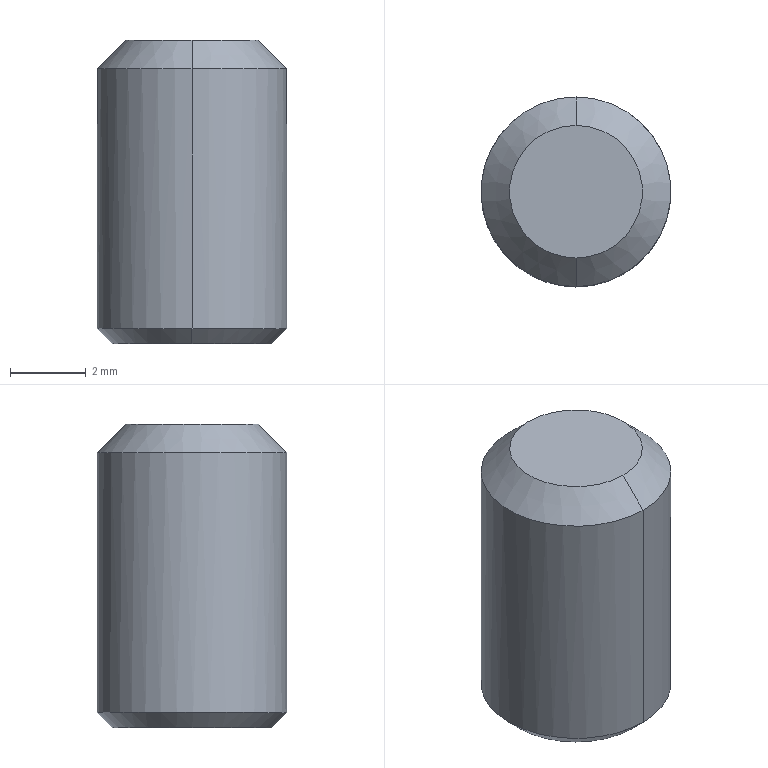Part | SolidWorks | features BaseBody 1 | 1 solid | 16 faces | box 5 x 5 x 8 mm | volume 135.67 mm3 | plane 10 | cone 4 | cylinder 2 | commonest cylinder face diameters 5 x2
STEP:
#1=CARTESIAN_POINT('',(483.507,-62.377,246.119));
#2=VERTEX_POINT('',#1);
#3=CARTESIAN_POINT('',(484.706,-62.684,246.118));
#4=VERTEX_POINT('',#3);
#5=CARTESIAN_POINT('',(483.507,-64.877,246.119));
#6=DIRECTION('',(-0.000000004,0.000000009,-1.));
#7=DIRECTION('',(0.,-1.,-0.000000009));
#8=AXIS2_PLACEMENT_3D('',#5,#6,#7);
#9=CIRCLE('',#8,2.5);
#10=EDGE_CURVE('',#2,#4,#9,.T.);
#11=ORIENTED_EDGE('',*,*,#10,.F.);
#12=CARTESIAN_POINT('',(483.507,-62.377,252.968));
#13=VERTEX_POINT('',#12);
#14=CARTESIAN_POINT('',(483.507,-62.377,249.543));
#15=DIRECTION('',(0.000000004,-0.000000009,1.));
#16=VECTOR('',#15,1000.);
#17=LINE('',#14,#16);
#18=EDGE_CURVE('',#2,#13,#17,.T.);
#19=ORIENTED_EDGE('',*,*,#18,.T.);
#20=CARTESIAN_POINT('',(483.507,-67.377,252.968));
#21=VERTEX_POINT('',#20);
#22=CARTESIAN_POINT('',(483.507,-64.877,252.968));
#23=DIRECTION('',(-0.000000004,0.000000009,-1.));
#24=DIRECTION('',(0.,-1.,-0.000000009));
#25=AXIS2_PLACEMENT_3D('',#22,#23,#24);
#26=CIRCLE('',#25,2.5);
#27=EDGE_CURVE('',#13,#21,#26,.T.);
#28=ORIENTED_EDGE('',*,*,#27,.T.);
#29=CARTESIAN_POINT('',(483.507,-67.377,246.118));
#30=VERTEX_POINT('',#29);
#31=CARTESIAN_POINT('',(483.507,-67.377,249.543));
#32=DIRECTION('',(0.000000004,-0.000000009,1.));
#33=VECTOR('',#32,1000.);
#34=LINE('',#31,#33);
#35=EDGE_CURVE('',#30,#21,#34,.T.);
#36=ORIENTED_EDGE('',*,*,#35,.F.);
#37=CARTESIAN_POINT('',(483.507,-64.877,246.118));
#38=DIRECTION('',(0.000000004,-0.000000009,1.));
#39=DIRECTION('',(0.,-1.,-0.000000009));
#40=AXIS2_PLACEMENT_3D('',#37,#38,#39);
#41=CIRCLE('',#40,2.5);
#42=EDGE_CURVE('',#30,#4,#41,.T.);
#43=ORIENTED_EDGE('',*,*,#42,.T.);
#44=EDGE_LOOP('',(#11,#19,#28,#36,#43));
#45=FACE_OUTER_BOUND('',#44,.T.);
#46=CARTESIAN_POINT('',(483.507,-64.877,249.543));
#47=DIRECTION('',(0.000000004,-0.000000009,1.));
#48=DIRECTION('',(0.,-1.,-0.000000009));
#49=AXIS2_PLACEMENT_3D('',#46,#47,#48);
#50=CYLINDRICAL_SURFACE('',#49,2.5);
#51=ADVANCED_FACE('',(#45),#50,.T.);
#52=CARTESIAN_POINT('',(483.507,-63.127,253.718));
#53=VERTEX_POINT('',#52);
#54=CARTESIAN_POINT('',(483.507,-66.627,253.718));
#55=VERTEX_POINT('',#54);
#56=CARTESIAN_POINT('',(483.507,-64.877,253.718));
#57=DIRECTION('',(-0.000000004,0.000000009,-1.));
#58=DIRECTION('',(0.,1.,0.000000009));
#59=AXIS2_PLACEMENT_3D('',#56,#57,#58);
#60=CIRCLE('',#59,1.75);
#61=EDGE_CURVE('',#53,#55,#60,.T.);
#62=ORIENTED_EDGE('',*,*,#61,.T.);
#63=CARTESIAN_POINT('',(483.507,-67.377,252.968));
#64=DIRECTION('',(-0.000000003,-0.7071,-0.7071));
#65=VECTOR('',#64,1000.);
#66=LINE('',#63,#65);
#67=EDGE_CURVE('',#55,#21,#66,.T.);
#68=ORIENTED_EDGE('',*,*,#67,.T.);
#69=ORIENTED_EDGE('',*,*,#27,.F.);
#70=CARTESIAN_POINT('',(483.507,-62.377,252.968));
#71=DIRECTION('',(-0.000000003,0.7071,-0.7071));
#72=VECTOR('',#71,1000.);
#73=LINE('',#70,#72);
#74=EDGE_CURVE('',#53,#13,#73,.T.);
#75=ORIENTED_EDGE('',*,*,#74,.F.);
#76=EDGE_LOOP('',(#62,#68,#69,#75));
#77=FACE_OUTER_BOUND('',#76,.T.);
#78=CARTESIAN_POINT('',(483.507,-64.877,252.968));
#79=DIRECTION('',(-0.000000004,0.000000009,-1.));
#80=DIRECTION('',(0.,1.,0.000000009));
#81=AXIS2_PLACEMENT_3D('',#78,#79,#80);
#82=CONICAL_SURFACE('',#81,2.5,0.7854);
#83=ADVANCED_FACE('',(#77),#82,.T.);
#84=CARTESIAN_POINT('',(483.507,-66.977,245.718));
#85=VERTEX_POINT('',#84);
#86=CARTESIAN_POINT('',(483.507,-62.777,245.718));
#87=VERTEX_POINT('',#86);
#88=CARTESIAN_POINT('',(483.507,-64.877,245.718));
#89=DIRECTION('',(0.000000004,-0.000000009,1.));
#90=DIRECTION('',(0.,-1.,-0.000000009));
#91=AXIS2_PLACEMENT_3D('',#88,#89,#90);
#92=CIRCLE('',#91,2.1);
#93=EDGE_CURVE('',#85,#87,#92,.T.);
#94=ORIENTED_EDGE('',*,*,#93,.T.);
#95=CARTESIAN_POINT('',(483.507,-62.378,246.118));
#96=DIRECTION('',(0.000000003,0.706,0.7082));
#97=VECTOR('',#96,1000.);
#98=LINE('',#95,#97);
#99=EDGE_CURVE('',#87,#2,#98,.T.);
#100=ORIENTED_EDGE('',*,*,#99,.T.);
#101=ORIENTED_EDGE('',*,*,#10,.T.);
#102=CARTESIAN_POINT('',(483.507,-67.376,246.118));
#103=VERTEX_POINT('',#102);
#104=CARTESIAN_POINT('',(483.507,-64.877,246.118));
#105=DIRECTION('',(0.000000004,-0.000000009,1.));
#106=DIRECTION('',(0.,-1.,-0.000000009));
#107=AXIS2_PLACEMENT_3D('',#104,#105,#106);
#108=CIRCLE('',#107,2.499);
#109=EDGE_CURVE('',#103,#4,#108,.T.);
#110=ORIENTED_EDGE('',*,*,#109,.F.);
#111=CARTESIAN_POINT('',(483.507,-67.376,246.118));
#112=DIRECTION('',(0.000000003,-0.706,0.7082));
#113=VECTOR('',#112,1000.);
#114=LINE('',#111,#113);
#115=EDGE_CURVE('',#85,#103,#114,.T.);
#116=ORIENTED_EDGE('',*,*,#115,.F.);
#117=EDGE_LOOP('',(#94,#100,#101,#110,#116));
#118=FACE_OUTER_BOUND('',#117,.T.);
#119=CARTESIAN_POINT('',(483.507,-64.877,246.118));
#120=DIRECTION('',(0.000000004,-0.000000009,1.));
#121=DIRECTION('',(0.,-1.,-0.000000009));
#122=AXIS2_PLACEMENT_3D('',#119,#120,#121);
#123=CONICAL_SURFACE('',#122,2.499,0.7838);
#124=ADVANCED_FACE('',(#118),#123,.T.);
#125=ORIENTED_EDGE('',*,*,#18,.F.);
#126=CARTESIAN_POINT('',(482.307,-67.07,246.118));
#127=VERTEX_POINT('',#126);
#128=CARTESIAN_POINT('',(483.507,-64.877,246.119));
#129=DIRECTION('',(-0.000000004,0.000000009,-1.));
#130=DIRECTION('',(0.,-1.,-0.000000009));
#131=AXIS2_PLACEMENT_3D('',#128,#129,#130);
#132=CIRCLE('',#131,2.5);
#133=EDGE_CURVE('',#127,#2,#132,.T.);
#134=ORIENTED_EDGE('',*,*,#133,.F.);
#135=CARTESIAN_POINT('',(483.507,-64.877,246.118));
#136=DIRECTION('',(0.000000004,-0.000000009,1.));
#137=DIRECTION('',(0.,-1.,-0.000000009));
#138=AXIS2_PLACEMENT_3D('',#135,#136,#137);
#139=CIRCLE('',#138,2.5);
#140=EDGE_CURVE('',#127,#30,#139,.T.);
#141=ORIENTED_EDGE('',*,*,#140,.T.);
#142=ORIENTED_EDGE('',*,*,#35,.T.);
#143=CARTESIAN_POINT('',(483.507,-64.877,252.968));
#144=DIRECTION('',(-0.000000004,0.000000009,-1.));
#145=DIRECTION('',(0.,-1.,-0.000000009));
#146=AXIS2_PLACEMENT_3D('',#143,#144,#145);
#147=CIRCLE('',#146,2.5);
#148=EDGE_CURVE('',#21,#13,#147,.T.);
#149=ORIENTED_EDGE('',*,*,#148,.T.);
#150=EDGE_LOOP('',(#125,#134,#141,#142,#149));
#151=FACE_OUTER_BOUND('',#150,.T.);
#152=CARTESIAN_POINT('',(483.507,-64.877,249.543));
#153=DIRECTION('',(0.000000004,-0.000000009,1.));
#154=DIRECTION('',(0.,-1.,-0.000000009));
#155=AXIS2_PLACEMENT_3D('',#152,#153,#154);
#156=CYLINDRICAL_SURFACE('',#155,2.5);
#157=ADVANCED_FACE('',(#151),#156,.T.);
#158=ORIENTED_EDGE('',*,*,#67,.F.);
#159=CARTESIAN_POINT('',(483.507,-64.877,253.718));
#160=DIRECTION('',(-0.000000004,0.000000009,-1.));
#161=DIRECTION('',(0.,1.,0.000000009));
#162=AXIS2_PLACEMENT_3D('',#159,#160,#161);
#163=CIRCLE('',#162,1.75);
#164=EDGE_CURVE('',#55,#53,#163,.T.);
#165=ORIENTED_EDGE('',*,*,#164,.T.);
#166=ORIENTED_EDGE('',*,*,#74,.T.);
#167=ORIENTED_EDGE('',*,*,#148,.F.);
#168=EDGE_LOOP('',(#158,#165,#166,#167));
#169=FACE_OUTER_BOUND('',#168,.T.);
#170=CARTESIAN_POINT('',(483.507,-64.877,252.968));
#171=DIRECTION('',(-0.000000004,0.000000009,-1.));
#172=DIRECTION('',(0.,1.,0.000000009));
#173=AXIS2_PLACEMENT_3D('',#170,#171,#172);
#174=CONICAL_SURFACE('',#173,2.5,0.7854);
#175=ADVANCED_FACE('',(#169),#174,.T.);
#176=ORIENTED_EDGE('',*,*,#140,.F.);
#177=CARTESIAN_POINT('',(483.507,-64.877,246.118));
#178=DIRECTION('',(0.000000004,-0.000000009,1.));
#179=DIRECTION('',(0.,-1.,-0.000000009));
#180=AXIS2_PLACEMENT_3D('',#177,#178,#179);
#181=CIRCLE('',#180,2.499);
#182=EDGE_CURVE('',#127,#103,#181,.T.);
#183=ORIENTED_EDGE('',*,*,#182,.T.);
#184=ORIENTED_EDGE('',*,*,#109,.T.);
#185=ORIENTED_EDGE('',*,*,#42,.F.);
#186=EDGE_LOOP('',(#176,#183,#184,#185));
#187=FACE_OUTER_BOUND('',#186,.T.);
#188=CARTESIAN_POINT('',(482.307,-67.07,246.118));
#189=DIRECTION('',(-0.000000004,0.000000009,-1.));
#190=DIRECTION('',(0.,1.,0.000000009));
#191=AXIS2_PLACEMENT_3D('',#188,#189,#190);
#192=PLANE('',#191);
#193=ADVANCED_FACE('',(#187),#192,.T.);
#194=ORIENTED_EDGE('',*,*,#61,.F.);
#195=ORIENTED_EDGE('',*,*,#164,.F.);
#196=EDGE_LOOP('',(#194,#195));
#197=FACE_OUTER_BOUND('',#196,.T.);
#198=CARTESIAN_POINT('',(483.087,-65.645,253.718));
#199=DIRECTION('',(0.000000004,-0.000000009,1.));
#200=DIRECTION('',(0.,-1.,-0.000000009));
#201=AXIS2_PLACEMENT_3D('',#198,#199,#200);
#202=PLANE('',#201);
#203=ADVANCED_FACE('',(#197),#202,.T.);
#204=ORIENTED_EDGE('',*,*,#99,.F.);
#205=CARTESIAN_POINT('',(483.507,-64.877,245.718));
#206=DIRECTION('',(0.000000004,-0.000000009,1.));
#207=DIRECTION('',(0.,-1.,-0.000000009));
#208=AXIS2_PLACEMENT_3D('',#205,#206,#207);
#209=CIRCLE('',#208,2.1);
#210=EDGE_CURVE('',#87,#85,#209,.T.);
#211=ORIENTED_EDGE('',*,*,#210,.T.);
#212=ORIENTED_EDGE('',*,*,#115,.T.);
#213=ORIENTED_EDGE('',*,*,#182,.F.);
#214=ORIENTED_EDGE('',*,*,#133,.T.);
#215=EDGE_LOOP('',(#204,#211,#212,#213,#214));
#216=FACE_OUTER_BOUND('',#215,.T.);
#217=CARTESIAN_POINT('',(483.507,-64.877,246.118));
#218=DIRECTION('',(0.000000004,-0.000000009,1.));
#219=DIRECTION('',(0.,-1.,-0.000000009));
#220=AXIS2_PLACEMENT_3D('',#217,#218,#219);
#221=CONICAL_SURFACE('',#220,2.499,0.7838);
#222=ADVANCED_FACE('',(#216),#221,.T.);
#223=ORIENTED_EDGE('',*,*,#93,.F.);
#224=ORIENTED_EDGE('',*,*,#210,.F.);
#225=EDGE_LOOP('',(#223,#224));
#226=FACE_OUTER_BOUND('',#225,.T.);
#227=CARTESIAN_POINT('',(484.95,-64.844,245.718));
#228=VERTEX_POINT('',#227);
#229=CARTESIAN_POINT('',(484.2,-63.611,245.718));
#230=VERTEX_POINT('',#229);
#231=CARTESIAN_POINT('',(484.2,-63.611,245.718));
#232=DIRECTION('',(-0.5198,0.8543,0.));
#233=VECTOR('',#232,1000.);
#234=LINE('',#231,#233);
#235=EDGE_CURVE('',#228,#230,#234,.T.);
#236=ORIENTED_EDGE('',*,*,#235,.T.);
#237=CARTESIAN_POINT('',(482.757,-63.644,245.718));
#238=VERTEX_POINT('',#237);
#239=CARTESIAN_POINT('',(484.2,-63.611,245.718));
#240=DIRECTION('',(-0.9997,-0.02304,0.000000004));
#241=VECTOR('',#240,1000.);
#242=LINE('',#239,#241);
#243=EDGE_CURVE('',#230,#238,#242,.T.);
#244=ORIENTED_EDGE('',*,*,#243,.T.);
#245=CARTESIAN_POINT('',(482.064,-64.91,245.718));
#246=VERTEX_POINT('',#245);
#247=CARTESIAN_POINT('',(482.064,-64.91,245.718));
#248=DIRECTION('',(-0.4799,-0.8773,0.));
#249=VECTOR('',#248,1000.);
#250=LINE('',#247,#249);
#251=EDGE_CURVE('',#238,#246,#250,.T.);
#252=ORIENTED_EDGE('',*,*,#251,.T.);
#253=CARTESIAN_POINT('',(482.814,-66.143,245.718));
#254=VERTEX_POINT('',#253);
#255=CARTESIAN_POINT('',(482.814,-66.143,245.718));
#256=DIRECTION('',(0.5198,-0.8543,0.));
#257=VECTOR('',#256,1000.);
#258=LINE('',#255,#257);
#259=EDGE_CURVE('',#246,#254,#258,.T.);
#260=ORIENTED_EDGE('',*,*,#259,.T.);
#261=CARTESIAN_POINT('',(484.257,-66.11,245.718));
#262=VERTEX_POINT('',#261);
#263=CARTESIAN_POINT('',(484.257,-66.11,245.718));
#264=DIRECTION('',(0.9997,0.02304,0.));
#265=VECTOR('',#264,1000.);
#266=LINE('',#263,#265);
#267=EDGE_CURVE('',#254,#262,#266,.T.);
#268=ORIENTED_EDGE('',*,*,#267,.T.);
#269=CARTESIAN_POINT('',(484.95,-64.844,245.718));
#270=DIRECTION('',(0.4799,0.8773,0.));
#271=VECTOR('',#270,1000.);
#272=LINE('',#269,#271);
#273=EDGE_CURVE('',#262,#228,#272,.T.);
#274=ORIENTED_EDGE('',*,*,#273,.T.);
#275=EDGE_LOOP('',(#236,#244,#252,#260,#268,#274));
#276=FACE_BOUND('',#275,.T.);
#277=CARTESIAN_POINT('',(483.003,-65.798,245.718));
#278=DIRECTION('',(-0.000000004,0.000000009,-1.));
#279=DIRECTION('',(0.,1.,0.000000009));
#280=AXIS2_PLACEMENT_3D('',#277,#278,#279);
#281=PLANE('',#280);
#282=ADVANCED_FACE('',(#226,#276),#281,.T.);
#283=CARTESIAN_POINT('',(482.757,-63.644,248.718));
#284=VERTEX_POINT('',#283);
#285=CARTESIAN_POINT('',(482.757,-63.644,245.718));
#286=DIRECTION('',(0.,-0.000000009,1.));
#287=VECTOR('',#286,1000.);
#288=LINE('',#285,#287);
#289=EDGE_CURVE('',#238,#284,#288,.T.);
#290=ORIENTED_EDGE('',*,*,#289,.F.);
#291=ORIENTED_EDGE('',*,*,#243,.F.);
#292=CARTESIAN_POINT('',(484.2,-63.611,248.718));
#293=VERTEX_POINT('',#292);
#294=CARTESIAN_POINT('',(484.2,-63.611,245.718));
#295=DIRECTION('',(0.,0.000000009,-1.));
#296=VECTOR('',#295,1000.);
#297=LINE('',#294,#296);
#298=EDGE_CURVE('',#293,#230,#297,.T.);
#299=ORIENTED_EDGE('',*,*,#298,.F.);
#300=CARTESIAN_POINT('',(482.757,-63.644,248.718));
#301=DIRECTION('',(0.9997,0.02304,0.));
#302=VECTOR('',#301,1000.);
#303=LINE('',#300,#302);
#304=EDGE_CURVE('',#284,#293,#303,.T.);
#305=ORIENTED_EDGE('',*,*,#304,.F.);
#306=EDGE_LOOP('',(#290,#291,#299,#305));
#307=FACE_OUTER_BOUND('',#306,.T.);
#308=CARTESIAN_POINT('',(482.757,-63.644,245.718));
#309=DIRECTION('',(-0.02304,0.9997,0.000000009));
#310=DIRECTION('',(-0.9997,-0.02304,0.));
#311=AXIS2_PLACEMENT_3D('',#308,#309,#310);
#312=PLANE('',#311);
#313=ADVANCED_FACE('',(#307),#312,.F.);
#314=CARTESIAN_POINT('',(484.257,-66.11,248.718));
#315=VERTEX_POINT('',#314);
#316=CARTESIAN_POINT('',(482.814,-66.143,248.718));
#317=VERTEX_POINT('',#316);
#318=CARTESIAN_POINT('',(484.257,-66.11,248.718));
#319=DIRECTION('',(-0.9997,-0.02304,0.));
#320=VECTOR('',#319,1000.);
#321=LINE('',#318,#320);
#322=EDGE_CURVE('',#315,#317,#321,.T.);
#323=ORIENTED_EDGE('',*,*,#322,.T.);
#324=CARTESIAN_POINT('',(482.064,-64.91,248.718));
#325=VERTEX_POINT('',#324);
#326=CARTESIAN_POINT('',(482.814,-66.143,248.718));
#327=DIRECTION('',(-0.5198,0.8543,0.));
#328=VECTOR('',#327,1000.);
#329=LINE('',#326,#328);
#330=EDGE_CURVE('',#317,#325,#329,.T.);
#331=ORIENTED_EDGE('',*,*,#330,.T.);
#332=CARTESIAN_POINT('',(482.064,-64.91,248.718));
#333=DIRECTION('',(0.4799,0.8773,0.000000006));
#334=VECTOR('',#333,1000.);
#335=LINE('',#332,#334);
#336=EDGE_CURVE('',#325,#284,#335,.T.);
#337=ORIENTED_EDGE('',*,*,#336,.T.);
#338=ORIENTED_EDGE('',*,*,#304,.T.);
#339=CARTESIAN_POINT('',(484.95,-64.844,248.718));
#340=VERTEX_POINT('',#339);
#341=CARTESIAN_POINT('',(484.2,-63.611,248.718));
#342=DIRECTION('',(0.5198,-0.8543,-0.000000009));
#343=VECTOR('',#342,1000.);
#344=LINE('',#341,#343);
#345=EDGE_CURVE('',#293,#340,#344,.T.);
#346=ORIENTED_EDGE('',*,*,#345,.T.);
#347=CARTESIAN_POINT('',(484.95,-64.844,248.718));
#348=DIRECTION('',(-0.4799,-0.8773,0.));
#349=VECTOR('',#348,1000.);
#350=LINE('',#347,#349);
#351=EDGE_CURVE('',#340,#315,#350,.T.);
#352=ORIENTED_EDGE('',*,*,#351,.T.);
#353=EDGE_LOOP('',(#323,#331,#337,#338,#346,#352));
#354=FACE_OUTER_BOUND('',#353,.T.);
#355=CARTESIAN_POINT('',(483.507,-64.877,248.718));
#356=DIRECTION('',(-0.000000004,0.000000009,-1.));
#357=DIRECTION('',(0.,1.,0.000000009));
#358=AXIS2_PLACEMENT_3D('',#355,#356,#357);
#359=PLANE('',#358);
#360=ADVANCED_FACE('',(#354),#359,.T.);
#361=CARTESIAN_POINT('',(482.064,-64.91,245.718));
#362=DIRECTION('',(0.000000007,-0.000000004,1.));
#363=VECTOR('',#362,1000.);
#364=LINE('',#361,#363);
#365=EDGE_CURVE('',#246,#325,#364,.T.);
#366=ORIENTED_EDGE('',*,*,#365,.F.);
#367=ORIENTED_EDGE('',*,*,#251,.F.);
#368=ORIENTED_EDGE('',*,*,#289,.T.);
#369=ORIENTED_EDGE('',*,*,#336,.F.);
#370=EDGE_LOOP('',(#366,#367,#368,#369));
#371=FACE_OUTER_BOUND('',#370,.T.);
#372=CARTESIAN_POINT('',(482.064,-64.91,245.718));
#373=DIRECTION('',(-0.8773,0.4799,0.000000008));
#374=DIRECTION('',(-0.4799,-0.8773,0.));
#375=AXIS2_PLACEMENT_3D('',#372,#373,#374);
#376=PLANE('',#375);
#377=ADVANCED_FACE('',(#371),#376,.F.);
#378=ORIENTED_EDGE('',*,*,#298,.T.);
#379=ORIENTED_EDGE('',*,*,#235,.F.);
#380=CARTESIAN_POINT('',(484.95,-64.844,245.718));
#381=DIRECTION('',(0.000000001,0.000000001,-1.));
#382=VECTOR('',#381,1000.);
#383=LINE('',#380,#382);
#384=EDGE_CURVE('',#340,#228,#383,.T.);
#385=ORIENTED_EDGE('',*,*,#384,.F.);
#386=ORIENTED_EDGE('',*,*,#345,.F.);
#387=EDGE_LOOP('',(#378,#379,#385,#386));
#388=FACE_OUTER_BOUND('',#387,.T.);
#389=CARTESIAN_POINT('',(484.2,-63.611,245.718));
#390=DIRECTION('',(0.8543,0.5198,0.000000001));
#391=DIRECTION('',(-0.5198,0.8543,0.));
#392=AXIS2_PLACEMENT_3D('',#389,#390,#391);
#393=PLANE('',#392);
#394=ADVANCED_FACE('',(#388),#393,.F.);
#395=CARTESIAN_POINT('',(482.814,-66.143,245.718));
#396=DIRECTION('',(-0.000000001,-0.000000001,1.));
#397=VECTOR('',#396,1000.);
#398=LINE('',#395,#397);
#399=EDGE_CURVE('',#254,#317,#398,.T.);
#400=ORIENTED_EDGE('',*,*,#399,.F.);
#401=ORIENTED_EDGE('',*,*,#259,.F.);
#402=ORIENTED_EDGE('',*,*,#365,.T.);
#403=ORIENTED_EDGE('',*,*,#330,.F.);
#404=EDGE_LOOP('',(#400,#401,#402,#403));
#405=FACE_OUTER_BOUND('',#404,.T.);
#406=CARTESIAN_POINT('',(482.814,-66.143,245.718));
#407=DIRECTION('',(-0.8543,-0.5198,-0.000000001));
#408=DIRECTION('',(0.5198,-0.8543,0.));
#409=AXIS2_PLACEMENT_3D('',#406,#407,#408);
#410=PLANE('',#409);
#411=ADVANCED_FACE('',(#405),#410,.F.);
#412=ORIENTED_EDGE('',*,*,#384,.T.);
#413=ORIENTED_EDGE('',*,*,#273,.F.);
#414=CARTESIAN_POINT('',(484.257,-66.11,245.718));
#415=DIRECTION('',(-0.000000007,0.000000004,-1.));
#416=VECTOR('',#415,1000.);
#417=LINE('',#414,#416);
#418=EDGE_CURVE('',#315,#262,#417,.T.);
#419=ORIENTED_EDGE('',*,*,#418,.F.);
#420=ORIENTED_EDGE('',*,*,#351,.F.);
#421=EDGE_LOOP('',(#412,#413,#419,#420));
#422=FACE_OUTER_BOUND('',#421,.T.);
#423=CARTESIAN_POINT('',(484.95,-64.844,245.718));
#424=DIRECTION('',(0.8773,-0.4799,-0.000000008));
#425=DIRECTION('',(0.4799,0.8773,0.));
#426=AXIS2_PLACEMENT_3D('',#423,#424,#425);
#427=PLANE('',#426);
#428=ADVANCED_FACE('',(#422),#427,.F.);
#429=ORIENTED_EDGE('',*,*,#418,.T.);
#430=ORIENTED_EDGE('',*,*,#267,.F.);
#431=ORIENTED_EDGE('',*,*,#399,.T.);
#432=ORIENTED_EDGE('',*,*,#322,.F.);
#433=EDGE_LOOP('',(#429,#430,#431,#432));
#434=FACE_OUTER_BOUND('',#433,.T.);
#435=CARTESIAN_POINT('',(484.257,-66.11,245.718));
#436=DIRECTION('',(0.02304,-0.9997,-0.000000009));
#437=DIRECTION('',(0.9997,0.02304,0.));
#438=AXIS2_PLACEMENT_3D('',#435,#436,#437);
#439=PLANE('',#438);
#440=ADVANCED_FACE('',(#434),#439,.F.);
#441=CLOSED_SHELL('',(#51,#83,#124,#157,#175,#193,#203,#222,#282,#313,#360,#377,#394,#411,#428,#440));
#442=MANIFOLD_SOLID_BREP('',#441);
#443=CARTESIAN_POINT('',(0.,0.,0.));
#444=DIRECTION('',(0.,0.,1.));
#445=DIRECTION('',(1.,0.,0.));
#446=AXIS2_PLACEMENT_3D('',#443,#444,#445);
#447=(LENGTH_UNIT()NAMED_UNIT(*)SI_UNIT(.MILLI.,.METRE.));
#448=UNCERTAINTY_MEASURE_WITH_UNIT(LENGTH_MEASURE(0.00001),#447,'','');
#449=(NAMED_UNIT(*)PLANE_ANGLE_UNIT()SI_UNIT($,.RADIAN.));
#450=(NAMED_UNIT(*)SI_UNIT($,.STERADIAN.)SOLID_ANGLE_UNIT());
#451=(GEOMETRIC_REPRESENTATION_CONTEXT(3)GLOBAL_UNCERTAINTY_ASSIGNED_CONTEXT((#448))GLOBAL_UNIT_ASSIGNED_CONTEXT((#447,#449,#450))REPRESENTATION_CONTEXT('',''));
#452=ADVANCED_BREP_SHAPE_REPRESENTATION('',(#442,#446),#451);